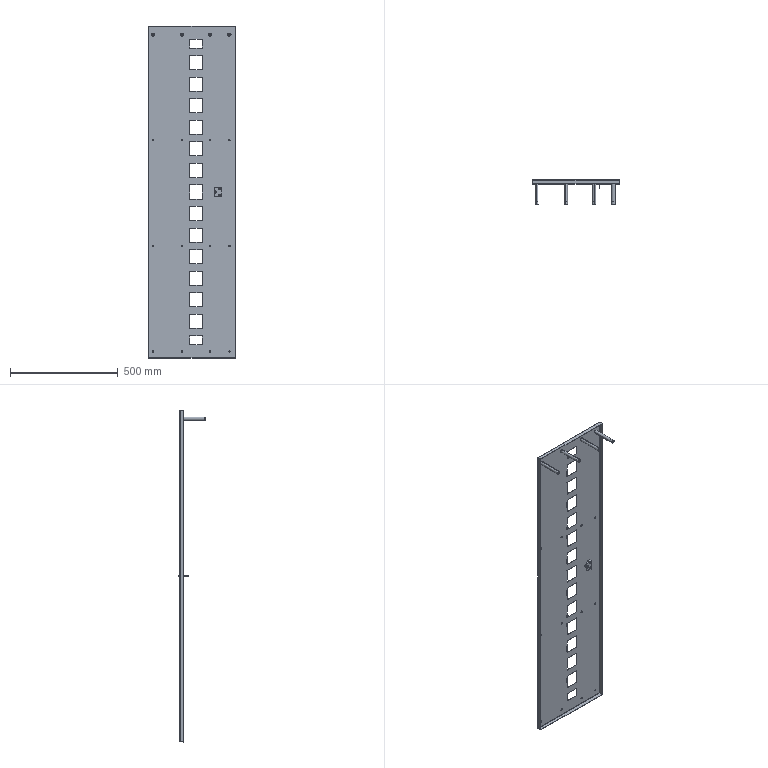Part | SolidWorks | 9 solids | 261 faces | box 407 x 121.237 x 1540 mm | volume 1039556 mm3 | plane 120 | cone 78 | cylinder 55 | spline 8 | commonest cylinder face diameters 5 x12 3.3 x8 15 x8 1.473 x4 4 x4 4.473 x4